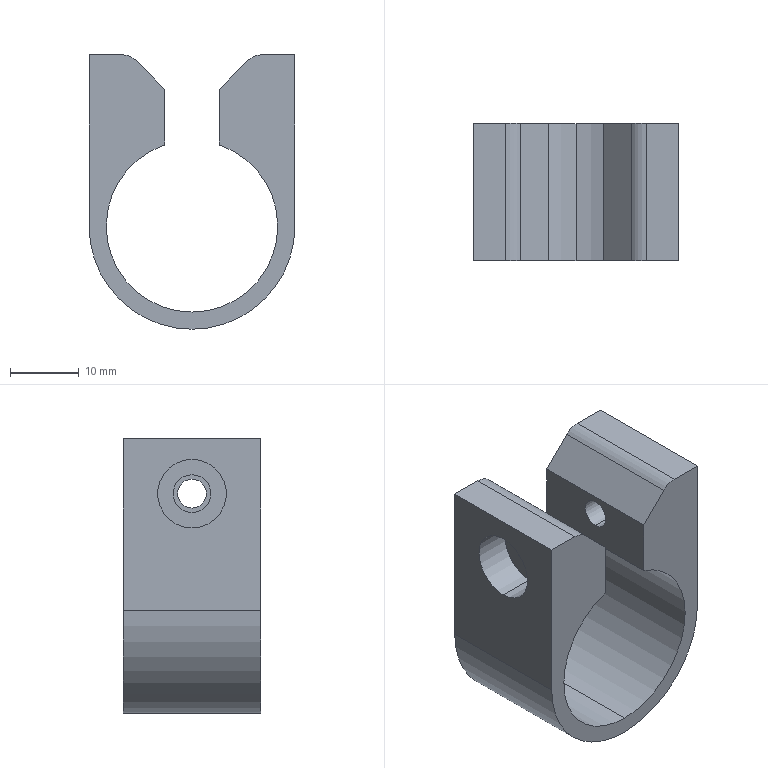Part | STEP file | Handlebar Clamp | 1 solid | 25 faces | box 30 x 20 x 40 mm | volume 8999 mm3 | cylinder 12 | plane 11 | cone 2 | commonest cylinder face diameters 4.2 x2 5.5 x2 6 x2 10 x2 25 x2 30 x2